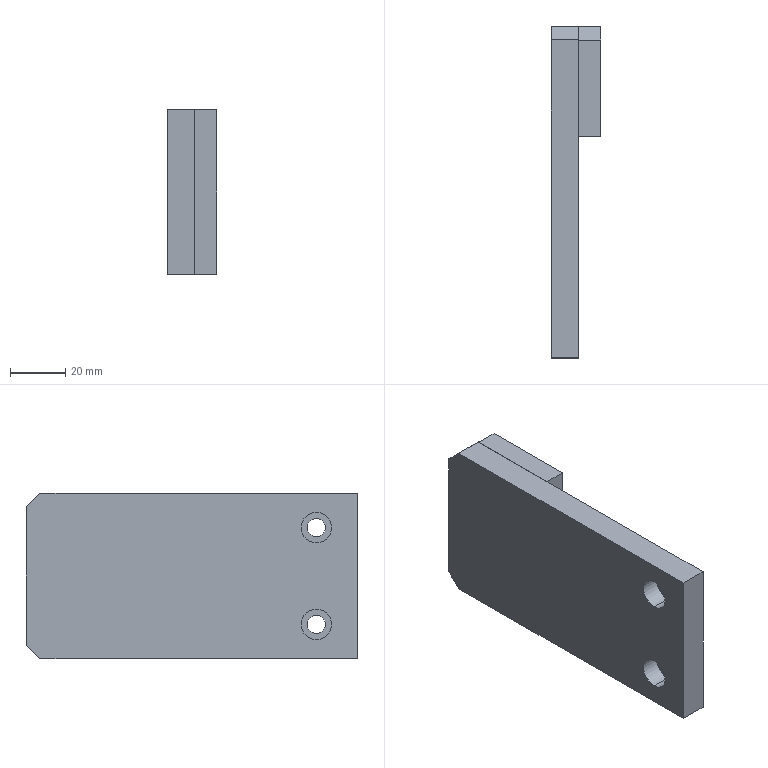Part | SolidWorks | features BaseBody 1 | 1 solid | 25 faces | box 18 x 120 x 60 mm | volume 89024 mm3 | plane 17 | cylinder 8 | commonest cylinder face diameters 6.6 x4 11 x4
STEP:
#1=CARTESIAN_POINT('',(6.8,15.,-23.));
#2=VERTEX_POINT('',#1);
#3=CARTESIAN_POINT('',(6.8,15.,-12.));
#4=VERTEX_POINT('',#3);
#5=CARTESIAN_POINT('',(6.8,15.,-17.5));
#6=DIRECTION('',(-1.,0.,0.));
#7=DIRECTION('',(0.,0.,1.));
#8=AXIS2_PLACEMENT_3D('',#5,#6,#7);
#9=CIRCLE('',#8,5.5);
#10=EDGE_CURVE('',#2,#4,#9,.T.);
#11=ORIENTED_EDGE('',*,*,#10,.F.);
#12=CARTESIAN_POINT('',(0.,15.,-23.));
#13=VERTEX_POINT('',#12);
#14=CARTESIAN_POINT('',(0.,15.,-23.));
#15=DIRECTION('',(-1.,0.,0.));
#16=VECTOR('',#15,1000.);
#17=LINE('',#14,#16);
#18=EDGE_CURVE('',#2,#13,#17,.T.);
#19=ORIENTED_EDGE('',*,*,#18,.T.);
#20=CARTESIAN_POINT('',(0.,15.,-12.));
#21=VERTEX_POINT('',#20);
#22=CARTESIAN_POINT('',(0.,15.,-17.5));
#23=DIRECTION('',(-1.,0.,0.));
#24=DIRECTION('',(0.,0.,1.));
#25=AXIS2_PLACEMENT_3D('',#22,#23,#24);
#26=CIRCLE('',#25,5.5);
#27=EDGE_CURVE('',#13,#21,#26,.T.);
#28=ORIENTED_EDGE('',*,*,#27,.T.);
#29=CARTESIAN_POINT('',(0.,15.,-12.));
#30=DIRECTION('',(-1.,0.,0.));
#31=VECTOR('',#30,1000.);
#32=LINE('',#29,#31);
#33=EDGE_CURVE('',#4,#21,#32,.T.);
#34=ORIENTED_EDGE('',*,*,#33,.F.);
#35=EDGE_LOOP('',(#11,#19,#28,#34));
#36=FACE_OUTER_BOUND('',#35,.T.);
#37=CARTESIAN_POINT('',(0.,15.,-17.5));
#38=DIRECTION('',(-1.,0.,0.));
#39=DIRECTION('',(0.,0.,1.));
#40=AXIS2_PLACEMENT_3D('',#37,#38,#39);
#41=CYLINDRICAL_SURFACE('',#40,5.5);
#42=ADVANCED_FACE('',(#36),#41,.F.);
#43=CARTESIAN_POINT('',(10.,15.,-20.8));
#44=VERTEX_POINT('',#43);
#45=CARTESIAN_POINT('',(10.,15.,-14.2));
#46=VERTEX_POINT('',#45);
#47=CARTESIAN_POINT('',(10.,15.,-17.5));
#48=DIRECTION('',(-1.,0.,0.));
#49=DIRECTION('',(0.,0.,1.));
#50=AXIS2_PLACEMENT_3D('',#47,#48,#49);
#51=CIRCLE('',#50,3.3);
#52=EDGE_CURVE('',#44,#46,#51,.T.);
#53=ORIENTED_EDGE('',*,*,#52,.F.);
#54=CARTESIAN_POINT('',(6.8,15.,-20.8));
#55=VERTEX_POINT('',#54);
#56=CARTESIAN_POINT('',(0.,15.,-20.8));
#57=DIRECTION('',(-1.,0.,0.));
#58=VECTOR('',#57,1000.);
#59=LINE('',#56,#58);
#60=EDGE_CURVE('',#44,#55,#59,.T.);
#61=ORIENTED_EDGE('',*,*,#60,.T.);
#62=CARTESIAN_POINT('',(6.8,15.,-14.2));
#63=VERTEX_POINT('',#62);
#64=CARTESIAN_POINT('',(6.8,15.,-17.5));
#65=DIRECTION('',(-1.,0.,0.));
#66=DIRECTION('',(0.,0.,1.));
#67=AXIS2_PLACEMENT_3D('',#64,#65,#66);
#68=CIRCLE('',#67,3.3);
#69=EDGE_CURVE('',#55,#63,#68,.T.);
#70=ORIENTED_EDGE('',*,*,#69,.T.);
#71=CARTESIAN_POINT('',(0.,15.,-14.2));
#72=DIRECTION('',(-1.,0.,0.));
#73=VECTOR('',#72,1000.);
#74=LINE('',#71,#73);
#75=EDGE_CURVE('',#46,#63,#74,.T.);
#76=ORIENTED_EDGE('',*,*,#75,.F.);
#77=EDGE_LOOP('',(#53,#61,#70,#76));
#78=FACE_OUTER_BOUND('',#77,.T.);
#79=CARTESIAN_POINT('',(0.,15.,-17.5));
#80=DIRECTION('',(-1.,0.,0.));
#81=DIRECTION('',(0.,0.,1.));
#82=AXIS2_PLACEMENT_3D('',#79,#80,#81);
#83=CYLINDRICAL_SURFACE('',#82,3.3);
#84=ADVANCED_FACE('',(#78),#83,.F.);
#85=CARTESIAN_POINT('',(6.8,15.,12.));
#86=VERTEX_POINT('',#85);
#87=CARTESIAN_POINT('',(6.8,15.,23.));
#88=VERTEX_POINT('',#87);
#89=CARTESIAN_POINT('',(6.8,15.,17.5));
#90=DIRECTION('',(-1.,0.,0.));
#91=DIRECTION('',(0.,0.,1.));
#92=AXIS2_PLACEMENT_3D('',#89,#90,#91);
#93=CIRCLE('',#92,5.5);
#94=EDGE_CURVE('',#86,#88,#93,.T.);
#95=ORIENTED_EDGE('',*,*,#94,.F.);
#96=CARTESIAN_POINT('',(0.,15.,12.));
#97=VERTEX_POINT('',#96);
#98=CARTESIAN_POINT('',(0.,15.,12.));
#99=DIRECTION('',(-1.,0.,0.));
#100=VECTOR('',#99,1000.);
#101=LINE('',#98,#100);
#102=EDGE_CURVE('',#86,#97,#101,.T.);
#103=ORIENTED_EDGE('',*,*,#102,.T.);
#104=CARTESIAN_POINT('',(0.,15.,23.));
#105=VERTEX_POINT('',#104);
#106=CARTESIAN_POINT('',(0.,15.,17.5));
#107=DIRECTION('',(-1.,0.,0.));
#108=DIRECTION('',(0.,0.,1.));
#109=AXIS2_PLACEMENT_3D('',#106,#107,#108);
#110=CIRCLE('',#109,5.5);
#111=EDGE_CURVE('',#97,#105,#110,.T.);
#112=ORIENTED_EDGE('',*,*,#111,.T.);
#113=CARTESIAN_POINT('',(0.,15.,23.));
#114=DIRECTION('',(-1.,0.,0.));
#115=VECTOR('',#114,1000.);
#116=LINE('',#113,#115);
#117=EDGE_CURVE('',#88,#105,#116,.T.);
#118=ORIENTED_EDGE('',*,*,#117,.F.);
#119=EDGE_LOOP('',(#95,#103,#112,#118));
#120=FACE_OUTER_BOUND('',#119,.T.);
#121=CARTESIAN_POINT('',(0.,15.,17.5));
#122=DIRECTION('',(-1.,0.,0.));
#123=DIRECTION('',(0.,0.,1.));
#124=AXIS2_PLACEMENT_3D('',#121,#122,#123);
#125=CYLINDRICAL_SURFACE('',#124,5.5);
#126=ADVANCED_FACE('',(#120),#125,.F.);
#127=CARTESIAN_POINT('',(10.,15.,14.2));
#128=VERTEX_POINT('',#127);
#129=CARTESIAN_POINT('',(10.,15.,20.8));
#130=VERTEX_POINT('',#129);
#131=CARTESIAN_POINT('',(10.,15.,17.5));
#132=DIRECTION('',(-1.,0.,0.));
#133=DIRECTION('',(0.,0.,1.));
#134=AXIS2_PLACEMENT_3D('',#131,#132,#133);
#135=CIRCLE('',#134,3.3);
#136=EDGE_CURVE('',#128,#130,#135,.T.);
#137=ORIENTED_EDGE('',*,*,#136,.F.);
#138=CARTESIAN_POINT('',(6.8,15.,14.2));
#139=VERTEX_POINT('',#138);
#140=CARTESIAN_POINT('',(0.,15.,14.2));
#141=DIRECTION('',(-1.,0.,0.));
#142=VECTOR('',#141,1000.);
#143=LINE('',#140,#142);
#144=EDGE_CURVE('',#128,#139,#143,.T.);
#145=ORIENTED_EDGE('',*,*,#144,.T.);
#146=CARTESIAN_POINT('',(6.8,15.,20.8));
#147=VERTEX_POINT('',#146);
#148=CARTESIAN_POINT('',(6.8,15.,17.5));
#149=DIRECTION('',(-1.,0.,0.));
#150=DIRECTION('',(0.,0.,1.));
#151=AXIS2_PLACEMENT_3D('',#148,#149,#150);
#152=CIRCLE('',#151,3.3);
#153=EDGE_CURVE('',#139,#147,#152,.T.);
#154=ORIENTED_EDGE('',*,*,#153,.T.);
#155=CARTESIAN_POINT('',(0.,15.,20.8));
#156=DIRECTION('',(-1.,0.,0.));
#157=VECTOR('',#156,1000.);
#158=LINE('',#155,#157);
#159=EDGE_CURVE('',#130,#147,#158,.T.);
#160=ORIENTED_EDGE('',*,*,#159,.F.);
#161=EDGE_LOOP('',(#137,#145,#154,#160));
#162=FACE_OUTER_BOUND('',#161,.T.);
#163=CARTESIAN_POINT('',(0.,15.,17.5));
#164=DIRECTION('',(-1.,0.,0.));
#165=DIRECTION('',(0.,0.,1.));
#166=AXIS2_PLACEMENT_3D('',#163,#164,#165);
#167=CYLINDRICAL_SURFACE('',#166,3.3);
#168=ADVANCED_FACE('',(#162),#167,.F.);
#169=CARTESIAN_POINT('',(18.,114.917,29.8));
#170=VERTEX_POINT('',#169);
#171=CARTESIAN_POINT('',(18.,80.,29.8));
#172=VERTEX_POINT('',#171);
#173=CARTESIAN_POINT('',(18.,114.917,29.8));
#174=DIRECTION('',(0.,-1.,0.));
#175=VECTOR('',#174,1000.);
#176=LINE('',#173,#175);
#177=EDGE_CURVE('',#170,#172,#176,.T.);
#178=ORIENTED_EDGE('',*,*,#177,.T.);
#179=CARTESIAN_POINT('',(18.,80.,-29.8));
#180=VERTEX_POINT('',#179);
#181=CARTESIAN_POINT('',(18.,80.,29.8));
#182=DIRECTION('',(0.,0.,-1.));
#183=VECTOR('',#182,1000.);
#184=LINE('',#181,#183);
#185=EDGE_CURVE('',#172,#180,#184,.T.);
#186=ORIENTED_EDGE('',*,*,#185,.T.);
#187=CARTESIAN_POINT('',(18.,114.917,-29.8));
#188=VERTEX_POINT('',#187);
#189=CARTESIAN_POINT('',(18.,80.,-29.8));
#190=DIRECTION('',(0.,1.,0.));
#191=VECTOR('',#190,1000.);
#192=LINE('',#189,#191);
#193=EDGE_CURVE('',#180,#188,#192,.T.);
#194=ORIENTED_EDGE('',*,*,#193,.T.);
#195=CARTESIAN_POINT('',(18.,119.8,-24.917));
#196=VERTEX_POINT('',#195);
#197=CARTESIAN_POINT('',(18.,114.917,-29.8));
#198=DIRECTION('',(0.,0.7071,0.7071));
#199=VECTOR('',#198,1000.);
#200=LINE('',#197,#199);
#201=EDGE_CURVE('',#188,#196,#200,.T.);
#202=ORIENTED_EDGE('',*,*,#201,.T.);
#203=CARTESIAN_POINT('',(18.,119.8,24.917));
#204=VERTEX_POINT('',#203);
#205=CARTESIAN_POINT('',(18.,119.8,-24.917));
#206=DIRECTION('',(0.,0.,1.));
#207=VECTOR('',#206,1000.);
#208=LINE('',#205,#207);
#209=EDGE_CURVE('',#196,#204,#208,.T.);
#210=ORIENTED_EDGE('',*,*,#209,.T.);
#211=CARTESIAN_POINT('',(18.,119.8,24.917));
#212=DIRECTION('',(0.,-0.7071,0.7071));
#213=VECTOR('',#212,1000.);
#214=LINE('',#211,#213);
#215=EDGE_CURVE('',#204,#170,#214,.T.);
#216=ORIENTED_EDGE('',*,*,#215,.T.);
#217=EDGE_LOOP('',(#178,#186,#194,#202,#210,#216));
#218=FACE_OUTER_BOUND('',#217,.T.);
#219=CARTESIAN_POINT('',(18.,0.,0.));
#220=DIRECTION('',(1.,0.,0.));
#221=DIRECTION('',(0.,1.,0.));
#222=AXIS2_PLACEMENT_3D('',#219,#220,#221);
#223=PLANE('',#222);
#224=ADVANCED_FACE('',(#218),#223,.T.);
#225=CARTESIAN_POINT('',(10.,119.8,24.917));
#226=VERTEX_POINT('',#225);
#227=CARTESIAN_POINT('',(10.,114.917,29.8));
#228=VERTEX_POINT('',#227);
#229=CARTESIAN_POINT('',(10.,119.8,24.917));
#230=DIRECTION('',(0.,-0.7071,0.7071));
#231=VECTOR('',#230,1000.);
#232=LINE('',#229,#231);
#233=EDGE_CURVE('',#226,#228,#232,.T.);
#234=ORIENTED_EDGE('',*,*,#233,.T.);
#235=CARTESIAN_POINT('',(18.,114.917,29.8));
#236=DIRECTION('',(-1.,0.,0.));
#237=VECTOR('',#236,1000.);
#238=LINE('',#235,#237);
#239=EDGE_CURVE('',#170,#228,#238,.T.);
#240=ORIENTED_EDGE('',*,*,#239,.F.);
#241=ORIENTED_EDGE('',*,*,#215,.F.);
#242=CARTESIAN_POINT('',(18.,119.8,24.917));
#243=DIRECTION('',(-1.,0.,0.));
#244=VECTOR('',#243,1000.);
#245=LINE('',#242,#244);
#246=EDGE_CURVE('',#204,#226,#245,.T.);
#247=ORIENTED_EDGE('',*,*,#246,.T.);
#248=EDGE_LOOP('',(#234,#240,#241,#247));
#249=FACE_OUTER_BOUND('',#248,.T.);
#250=CARTESIAN_POINT('',(18.,119.8,24.917));
#251=DIRECTION('',(0.,-0.7071,-0.7071));
#252=DIRECTION('',(0.,0.7071,-0.7071));
#253=AXIS2_PLACEMENT_3D('',#250,#251,#252);
#254=PLANE('',#253);
#255=ADVANCED_FACE('',(#249),#254,.F.);
#256=CARTESIAN_POINT('',(10.,119.8,-24.917));
#257=VERTEX_POINT('',#256);
#258=CARTESIAN_POINT('',(10.,119.8,-24.917));
#259=DIRECTION('',(0.,0.,1.));
#260=VECTOR('',#259,1000.);
#261=LINE('',#258,#260);
#262=EDGE_CURVE('',#257,#226,#261,.T.);
#263=ORIENTED_EDGE('',*,*,#262,.T.);
#264=ORIENTED_EDGE('',*,*,#246,.F.);
#265=ORIENTED_EDGE('',*,*,#209,.F.);
#266=CARTESIAN_POINT('',(18.,119.8,-24.917));
#267=DIRECTION('',(-1.,0.,0.));
#268=VECTOR('',#267,1000.);
#269=LINE('',#266,#268);
#270=EDGE_CURVE('',#196,#257,#269,.T.);
#271=ORIENTED_EDGE('',*,*,#270,.T.);
#272=EDGE_LOOP('',(#263,#264,#265,#271));
#273=FACE_OUTER_BOUND('',#272,.T.);
#274=CARTESIAN_POINT('',(18.,119.8,-24.917));
#275=DIRECTION('',(0.,-1.,0.));
#276=DIRECTION('',(0.,0.,-1.));
#277=AXIS2_PLACEMENT_3D('',#274,#275,#276);
#278=PLANE('',#277);
#279=ADVANCED_FACE('',(#273),#278,.F.);
#280=CARTESIAN_POINT('',(10.,114.917,-29.8));
#281=VERTEX_POINT('',#280);
#282=CARTESIAN_POINT('',(10.,114.917,-29.8));
#283=DIRECTION('',(0.,0.7071,0.7071));
#284=VECTOR('',#283,1000.);
#285=LINE('',#282,#284);
#286=EDGE_CURVE('',#281,#257,#285,.T.);
#287=ORIENTED_EDGE('',*,*,#286,.T.);
#288=ORIENTED_EDGE('',*,*,#270,.F.);
#289=ORIENTED_EDGE('',*,*,#201,.F.);
#290=CARTESIAN_POINT('',(18.,114.917,-29.8));
#291=DIRECTION('',(-1.,0.,0.));
#292=VECTOR('',#291,1000.);
#293=LINE('',#290,#292);
#294=EDGE_CURVE('',#188,#281,#293,.T.);
#295=ORIENTED_EDGE('',*,*,#294,.T.);
#296=EDGE_LOOP('',(#287,#288,#289,#295));
#297=FACE_OUTER_BOUND('',#296,.T.);
#298=CARTESIAN_POINT('',(18.,114.917,-29.8));
#299=DIRECTION('',(0.,-0.7071,0.7071));
#300=DIRECTION('',(-1.,0.,0.));
#301=AXIS2_PLACEMENT_3D('',#298,#299,#300);
#302=PLANE('',#301);
#303=ADVANCED_FACE('',(#297),#302,.F.);
#304=CARTESIAN_POINT('',(10.,80.,-29.8));
#305=VERTEX_POINT('',#304);
#306=CARTESIAN_POINT('',(10.,80.,-29.8));
#307=DIRECTION('',(0.,1.,0.));
#308=VECTOR('',#307,1000.);
#309=LINE('',#306,#308);
#310=EDGE_CURVE('',#305,#281,#309,.T.);
#311=ORIENTED_EDGE('',*,*,#310,.T.);
#312=ORIENTED_EDGE('',*,*,#294,.F.);
#313=ORIENTED_EDGE('',*,*,#193,.F.);
#314=CARTESIAN_POINT('',(18.,80.,-29.8));
#315=DIRECTION('',(-1.,0.,0.));
#316=VECTOR('',#315,1000.);
#317=LINE('',#314,#316);
#318=EDGE_CURVE('',#180,#305,#317,.T.);
#319=ORIENTED_EDGE('',*,*,#318,.T.);
#320=EDGE_LOOP('',(#311,#312,#313,#319));
#321=FACE_OUTER_BOUND('',#320,.T.);
#322=CARTESIAN_POINT('',(18.,80.,-29.8));
#323=DIRECTION('',(0.,0.,1.));
#324=DIRECTION('',(0.,-1.,0.));
#325=AXIS2_PLACEMENT_3D('',#322,#323,#324);
#326=PLANE('',#325);
#327=ADVANCED_FACE('',(#321),#326,.F.);
#328=CARTESIAN_POINT('',(10.,80.,29.8));
#329=VERTEX_POINT('',#328);
#330=CARTESIAN_POINT('',(10.,80.,29.8));
#331=DIRECTION('',(0.,0.,-1.));
#332=VECTOR('',#331,1000.);
#333=LINE('',#330,#332);
#334=EDGE_CURVE('',#329,#305,#333,.T.);
#335=ORIENTED_EDGE('',*,*,#334,.T.);
#336=ORIENTED_EDGE('',*,*,#318,.F.);
#337=ORIENTED_EDGE('',*,*,#185,.F.);
#338=CARTESIAN_POINT('',(18.,80.,29.8));
#339=DIRECTION('',(-1.,0.,0.));
#340=VECTOR('',#339,1000.);
#341=LINE('',#338,#340);
#342=EDGE_CURVE('',#172,#329,#341,.T.);
#343=ORIENTED_EDGE('',*,*,#342,.T.);
#344=EDGE_LOOP('',(#335,#336,#337,#343));
#345=FACE_OUTER_BOUND('',#344,.T.);
#346=CARTESIAN_POINT('',(18.,80.,29.8));
#347=DIRECTION('',(0.,1.,0.));
#348=DIRECTION('',(1.,0.,0.));
#349=AXIS2_PLACEMENT_3D('',#346,#347,#348);
#350=PLANE('',#349);
#351=ADVANCED_FACE('',(#345),#350,.F.);
#352=CARTESIAN_POINT('',(10.,114.917,29.8));
#353=DIRECTION('',(0.,-1.,0.));
#354=VECTOR('',#353,1000.);
#355=LINE('',#352,#354);
#356=EDGE_CURVE('',#228,#329,#355,.T.);
#357=ORIENTED_EDGE('',*,*,#356,.T.);
#358=ORIENTED_EDGE('',*,*,#342,.F.);
#359=ORIENTED_EDGE('',*,*,#177,.F.);
#360=ORIENTED_EDGE('',*,*,#239,.T.);
#361=EDGE_LOOP('',(#357,#358,#359,#360));
#362=FACE_OUTER_BOUND('',#361,.T.);
#363=CARTESIAN_POINT('',(18.,114.917,29.8));
#364=DIRECTION('',(0.,0.,-1.));
#365=DIRECTION('',(-1.,0.,0.));
#366=AXIS2_PLACEMENT_3D('',#363,#364,#365);
#367=PLANE('',#366);
#368=ADVANCED_FACE('',(#362),#367,.F.);
#369=CARTESIAN_POINT('',(10.,120.,25.));
#370=VERTEX_POINT('',#369);
#371=CARTESIAN_POINT('',(10.,115.,30.));
#372=VERTEX_POINT('',#371);
#373=CARTESIAN_POINT('',(10.,115.,30.));
#374=DIRECTION('',(0.,-0.7071,0.7071));
#375=VECTOR('',#374,1000.);
#376=LINE('',#373,#375);
#377=EDGE_CURVE('',#370,#372,#376,.T.);
#378=ORIENTED_EDGE('',*,*,#377,.F.);
#379=CARTESIAN_POINT('',(0.,120.,25.));
#380=VERTEX_POINT('',#379);
#381=CARTESIAN_POINT('',(10.,120.,25.));
#382=DIRECTION('',(1.,0.,0.));
#383=VECTOR('',#382,1000.);
#384=LINE('',#381,#383);
#385=EDGE_CURVE('',#380,#370,#384,.T.);
#386=ORIENTED_EDGE('',*,*,#385,.F.);
#387=CARTESIAN_POINT('',(0.,115.,30.));
#388=VERTEX_POINT('',#387);
#389=CARTESIAN_POINT('',(0.,72.5,72.5));
#390=DIRECTION('',(0.,0.7071,-0.7071));
#391=VECTOR('',#390,1000.);
#392=LINE('',#389,#391);
#393=EDGE_CURVE('',#388,#380,#392,.T.);
#394=ORIENTED_EDGE('',*,*,#393,.F.);
#395=CARTESIAN_POINT('',(10.,115.,30.));
#396=DIRECTION('',(-1.,0.,0.));
#397=VECTOR('',#396,1000.);
#398=LINE('',#395,#397);
#399=EDGE_CURVE('',#372,#388,#398,.T.);
#400=ORIENTED_EDGE('',*,*,#399,.F.);
#401=EDGE_LOOP('',(#378,#386,#394,#400));
#402=FACE_OUTER_BOUND('',#401,.T.);
#403=CARTESIAN_POINT('',(10.,115.,30.));
#404=DIRECTION('',(0.,-0.7071,-0.7071));
#405=DIRECTION('',(0.,0.7071,-0.7071));
#406=AXIS2_PLACEMENT_3D('',#403,#404,#405);
#407=PLANE('',#406);
#408=ADVANCED_FACE('',(#402),#407,.F.);
#409=CARTESIAN_POINT('',(10.,115.,-30.));
#410=VERTEX_POINT('',#409);
#411=CARTESIAN_POINT('',(10.,120.,-25.));
#412=VERTEX_POINT('',#411);
#413=CARTESIAN_POINT('',(10.,120.,-25.));
#414=DIRECTION('',(0.,0.7071,0.7071));
#415=VECTOR('',#414,1000.);
#416=LINE('',#413,#415);
#417=EDGE_CURVE('',#410,#412,#416,.T.);
#418=ORIENTED_EDGE('',*,*,#417,.F.);
#419=CARTESIAN_POINT('',(0.,115.,-30.));
#420=VERTEX_POINT('',#419);
#421=CARTESIAN_POINT('',(10.,115.,-30.));
#422=DIRECTION('',(1.,0.,0.));
#423=VECTOR('',#422,1000.);
#424=LINE('',#421,#423);
#425=EDGE_CURVE('',#420,#410,#424,.T.);
#426=ORIENTED_EDGE('',*,*,#425,.F.);
#427=CARTESIAN_POINT('',(0.,120.,-25.));
#428=VERTEX_POINT('',#427);
#429=CARTESIAN_POINT('',(0.,72.5,-72.5));
#430=DIRECTION('',(0.,-0.7071,-0.7071));
#431=VECTOR('',#430,1000.);
#432=LINE('',#429,#431);
#433=EDGE_CURVE('',#428,#420,#432,.T.);
#434=ORIENTED_EDGE('',*,*,#433,.F.);
#435=CARTESIAN_POINT('',(10.,120.,-25.));
#436=DIRECTION('',(-1.,0.,0.));
#437=VECTOR('',#436,1000.);
#438=LINE('',#435,#437);
#439=EDGE_CURVE('',#412,#428,#438,.T.);
#440=ORIENTED_EDGE('',*,*,#439,.F.);
#441=EDGE_LOOP('',(#418,#426,#434,#440));
#442=FACE_OUTER_BOUND('',#441,.T.);
#443=CARTESIAN_POINT('',(10.,120.,-25.));
#444=DIRECTION('',(0.,-0.7071,0.7071));
#445=DIRECTION('',(-1.,0.,0.));
#446=AXIS2_PLACEMENT_3D('',#443,#444,#445);
#447=PLANE('',#446);
#448=ADVANCED_FACE('',(#442),#447,.F.);
#449=CARTESIAN_POINT('',(6.8,15.,-17.5));
#450=DIRECTION('',(-1.,0.,0.));
#451=DIRECTION('',(0.,0.,1.));
#452=AXIS2_PLACEMENT_3D('',#449,#450,#451);
#453=CIRCLE('',#452,3.3);
#454=EDGE_CURVE('',#63,#55,#453,.T.);
#455=ORIENTED_EDGE('',*,*,#454,.F.);
#456=ORIENTED_EDGE('',*,*,#69,.F.);
#457=EDGE_LOOP('',(#455,#456));
#458=FACE_BOUND('',#457,.T.);
#459=CARTESIAN_POINT('',(6.8,15.,-17.5));
#460=DIRECTION('',(-1.,0.,0.));
#461=DIRECTION('',(0.,0.,1.));
#462=AXIS2_PLACEMENT_3D('',#459,#460,#461);
#463=CIRCLE('',#462,5.5);
#464=EDGE_CURVE('',#4,#2,#463,.T.);
#465=ORIENTED_EDGE('',*,*,#464,.T.);
#466=ORIENTED_EDGE('',*,*,#10,.T.);
#467=EDGE_LOOP('',(#465,#466));
#468=FACE_OUTER_BOUND('',#467,.T.);
#469=CARTESIAN_POINT('',(6.8,18.3,-17.5));
#470=DIRECTION('',(1.,0.,0.));
#471=DIRECTION('',(0.,1.,0.));
#472=AXIS2_PLACEMENT_3D('',#469,#470,#471);
#473=PLANE('',#472);
#474=ADVANCED_FACE('',(#458,#468),#473,.F.);
#475=CARTESIAN_POINT('',(6.8,15.,17.5));
#476=DIRECTION('',(-1.,0.,0.));
#477=DIRECTION('',(0.,0.,1.));
#478=AXIS2_PLACEMENT_3D('',#475,#476,#477);
#479=CIRCLE('',#478,3.3);
#480=EDGE_CURVE('',#147,#139,#479,.T.);
#481=ORIENTED_EDGE('',*,*,#480,.F.);
#482=ORIENTED_EDGE('',*,*,#153,.F.);
#483=EDGE_LOOP('',(#481,#482));
#484=FACE_BOUND('',#483,.T.);
#485=CARTESIAN_POINT('',(6.8,15.,17.5));
#486=DIRECTION('',(-1.,0.,0.));
#487=DIRECTION('',(0.,0.,1.));
#488=AXIS2_PLACEMENT_3D('',#485,#486,#487);
#489=CIRCLE('',#488,5.5);
#490=EDGE_CURVE('',#88,#86,#489,.T.);
#491=ORIENTED_EDGE('',*,*,#490,.T.);
#492=ORIENTED_EDGE('',*,*,#94,.T.);
#493=EDGE_LOOP('',(#491,#492));
#494=FACE_OUTER_BOUND('',#493,.T.);
#495=CARTESIAN_POINT('',(6.8,18.3,17.5));
#496=DIRECTION('',(1.,0.,0.));
#497=DIRECTION('',(0.,1.,0.));
#498=AXIS2_PLACEMENT_3D('',#495,#496,#497);
#499=PLANE('',#498);
#500=ADVANCED_FACE('',(#484,#494),#499,.F.);
#501=CARTESIAN_POINT('',(0.,15.,17.5));
#502=DIRECTION('',(-1.,0.,0.));
#503=DIRECTION('',(0.,0.,1.));
#504=AXIS2_PLACEMENT_3D('',#501,#502,#503);
#505=CIRCLE('',#504,5.5);
#506=EDGE_CURVE('',#105,#97,#505,.T.);
#507=ORIENTED_EDGE('',*,*,#506,.F.);
#508=ORIENTED_EDGE('',*,*,#111,.F.);
#509=EDGE_LOOP('',(#507,#508));
#510=FACE_BOUND('',#509,.T.);
#511=CARTESIAN_POINT('',(0.,15.,-17.5));
#512=DIRECTION('',(-1.,0.,0.));
#513=DIRECTION('',(0.,0.,1.));
#514=AXIS2_PLACEMENT_3D('',#511,#512,#513);
#515=CIRCLE('',#514,5.5);
#516=EDGE_CURVE('',#21,#13,#515,.T.);
#517=ORIENTED_EDGE('',*,*,#516,.F.);
#518=ORIENTED_EDGE('',*,*,#27,.F.);
#519=EDGE_LOOP('',(#517,#518));
#520=FACE_BOUND('',#519,.T.);
#521=CARTESIAN_POINT('',(0.,120.,30.));
#522=DIRECTION('',(0.,0.,1.));
#523=VECTOR('',#522,1000.);
#524=LINE('',#521,#523);
#525=EDGE_CURVE('',#428,#380,#524,.T.);
#526=ORIENTED_EDGE('',*,*,#525,.F.);
#527=ORIENTED_EDGE('',*,*,#433,.T.);
#528=CARTESIAN_POINT('',(0.,0.,-30.));
#529=VERTEX_POINT('',#528);
#530=CARTESIAN_POINT('',(0.,0.,-30.));
#531=DIRECTION('',(0.,1.,0.));
#532=VECTOR('',#531,1000.);
#533=LINE('',#530,#532);
#534=EDGE_CURVE('',#529,#420,#533,.T.);
#535=ORIENTED_EDGE('',*,*,#534,.F.);
#536=CARTESIAN_POINT('',(0.,0.,30.));
#537=VERTEX_POINT('',#536);
#538=CARTESIAN_POINT('',(0.,0.,30.));
#539=DIRECTION('',(0.,0.,-1.));
#540=VECTOR('',#539,1000.);
#541=LINE('',#538,#540);
#542=EDGE_CURVE('',#537,#529,#541,.T.);
#543=ORIENTED_EDGE('',*,*,#542,.F.);
#544=CARTESIAN_POINT('',(0.,0.,30.));
#545=DIRECTION('',(0.,-1.,0.));
#546=VECTOR('',#545,1000.);
#547=LINE('',#544,#546);
#548=EDGE_CURVE('',#388,#537,#547,.T.);
#549=ORIENTED_EDGE('',*,*,#548,.F.);
#550=ORIENTED_EDGE('',*,*,#393,.T.);
#551=EDGE_LOOP('',(#526,#527,#535,#543,#549,#550));
#552=FACE_OUTER_BOUND('',#551,.T.);
#553=CARTESIAN_POINT('',(0.,0.,0.));
#554=DIRECTION('',(-1.,0.,0.));
#555=DIRECTION('',(0.,0.,1.));
#556=AXIS2_PLACEMENT_3D('',#553,#554,#555);
#557=PLANE('',#556);
#558=ADVANCED_FACE('',(#510,#520,#552),#557,.T.);
#559=CARTESIAN_POINT('',(10.,120.,30.));
#560=DIRECTION('',(0.,0.,1.));
#561=VECTOR('',#560,1000.);
#562=LINE('',#559,#561);
#563=EDGE_CURVE('',#412,#370,#562,.T.);
#564=ORIENTED_EDGE('',*,*,#563,.F.);
#565=ORIENTED_EDGE('',*,*,#439,.T.);
#566=ORIENTED_EDGE('',*,*,#525,.T.);
#567=ORIENTED_EDGE('',*,*,#385,.T.);
#568=EDGE_LOOP('',(#564,#565,#566,#567));
#569=FACE_OUTER_BOUND('',#568,.T.);
#570=CARTESIAN_POINT('',(10.,120.,30.));
#571=DIRECTION('',(0.,-1.,0.));
#572=DIRECTION('',(0.,0.,-1.));
#573=AXIS2_PLACEMENT_3D('',#570,#571,#572);
#574=PLANE('',#573);
#575=ADVANCED_FACE('',(#569),#574,.F.);
#576=ORIENTED_EDGE('',*,*,#534,.T.);
#577=ORIENTED_EDGE('',*,*,#425,.T.);
#578=CARTESIAN_POINT('',(10.,0.,-30.));
#579=VERTEX_POINT('',#578);
#580=CARTESIAN_POINT('',(10.,0.,-30.));
#581=DIRECTION('',(0.,1.,0.));
#582=VECTOR('',#581,1000.);
#583=LINE('',#580,#582);
#584=EDGE_CURVE('',#579,#410,#583,.T.);
#585=ORIENTED_EDGE('',*,*,#584,.F.);
#586=CARTESIAN_POINT('',(10.,0.,-30.));
#587=DIRECTION('',(-1.,0.,0.));
#588=VECTOR('',#587,1000.);
#589=LINE('',#586,#588);
#590=EDGE_CURVE('',#579,#529,#589,.T.);
#591=ORIENTED_EDGE('',*,*,#590,.T.);
#592=EDGE_LOOP('',(#576,#577,#585,#591));
#593=FACE_OUTER_BOUND('',#592,.T.);
#594=CARTESIAN_POINT('',(10.,0.,-30.));
#595=DIRECTION('',(0.,0.,1.));
#596=DIRECTION('',(1.,0.,0.));
#597=AXIS2_PLACEMENT_3D('',#594,#595,#596);
#598=PLANE('',#597);
#599=ADVANCED_FACE('',(#593),#598,.F.);
#600=ORIENTED_EDGE('',*,*,#542,.T.);
#601=ORIENTED_EDGE('',*,*,#590,.F.);
#602=CARTESIAN_POINT('',(10.,0.,30.));
#603=VERTEX_POINT('',#602);
#604=CARTESIAN_POINT('',(10.,0.,30.));
#605=DIRECTION('',(0.,0.,-1.));
#606=VECTOR('',#605,1000.);
#607=LINE('',#604,#606);
#608=EDGE_CURVE('',#603,#579,#607,.T.);
#609=ORIENTED_EDGE('',*,*,#608,.F.);
#610=CARTESIAN_POINT('',(10.,0.,30.));
#611=DIRECTION('',(-1.,0.,0.));
#612=VECTOR('',#611,1000.);
#613=LINE('',#610,#612);
#614=EDGE_CURVE('',#603,#537,#613,.T.);
#615=ORIENTED_EDGE('',*,*,#614,.T.);
#616=EDGE_LOOP('',(#600,#601,#609,#615));
#617=FACE_OUTER_BOUND('',#616,.T.);
#618=CARTESIAN_POINT('',(10.,0.,30.));
#619=DIRECTION('',(0.,1.,0.));
#620=DIRECTION('',(1.,0.,0.));
#621=AXIS2_PLACEMENT_3D('',#618,#619,#620);
#622=PLANE('',#621);
#623=ADVANCED_FACE('',(#617),#622,.F.);
#624=CARTESIAN_POINT('',(10.,0.,30.));
#625=DIRECTION('',(0.,-1.,0.));
#626=VECTOR('',#625,1000.);
#627=LINE('',#624,#626);
#628=EDGE_CURVE('',#372,#603,#627,.T.);
#629=ORIENTED_EDGE('',*,*,#628,.F.);
#630=ORIENTED_EDGE('',*,*,#399,.T.);
#631=ORIENTED_EDGE('',*,*,#548,.T.);
#632=ORIENTED_EDGE('',*,*,#614,.F.);
#633=EDGE_LOOP('',(#629,#630,#631,#632));
#634=FACE_OUTER_BOUND('',#633,.T.);
#635=CARTESIAN_POINT('',(10.,0.,30.));
#636=DIRECTION('',(0.,0.,-1.));
#637=DIRECTION('',(0.,-1.,0.));
#638=AXIS2_PLACEMENT_3D('',#635,#636,#637);
#639=PLANE('',#638);
#640=ADVANCED_FACE('',(#634),#639,.F.);
#641=ORIENTED_EDGE('',*,*,#356,.F.);
#642=ORIENTED_EDGE('',*,*,#233,.F.);
#643=ORIENTED_EDGE('',*,*,#262,.F.);
#644=ORIENTED_EDGE('',*,*,#286,.F.);
#645=ORIENTED_EDGE('',*,*,#310,.F.);
#646=ORIENTED_EDGE('',*,*,#334,.F.);
#647=EDGE_LOOP('',(#641,#642,#643,#644,#645,#646));
#648=FACE_BOUND('',#647,.T.);
#649=CARTESIAN_POINT('',(10.,15.,-17.5));
#650=DIRECTION('',(-1.,0.,0.));
#651=DIRECTION('',(0.,0.,1.));
#652=AXIS2_PLACEMENT_3D('',#649,#650,#651);
#653=CIRCLE('',#652,3.3);
#654=EDGE_CURVE('',#46,#44,#653,.T.);
#655=ORIENTED_EDGE('',*,*,#654,.T.);
#656=ORIENTED_EDGE('',*,*,#52,.T.);
#657=EDGE_LOOP('',(#655,#656));
#658=FACE_BOUND('',#657,.T.);
#659=CARTESIAN_POINT('',(10.,15.,17.5));
#660=DIRECTION('',(-1.,0.,0.));
#661=DIRECTION('',(0.,0.,1.));
#662=AXIS2_PLACEMENT_3D('',#659,#660,#661);
#663=CIRCLE('',#662,3.3);
#664=EDGE_CURVE('',#130,#128,#663,.T.);
#665=ORIENTED_EDGE('',*,*,#664,.T.);
#666=ORIENTED_EDGE('',*,*,#136,.T.);
#667=EDGE_LOOP('',(#665,#666));
#668=FACE_BOUND('',#667,.T.);
#669=ORIENTED_EDGE('',*,*,#584,.T.);
#670=ORIENTED_EDGE('',*,*,#417,.T.);
#671=ORIENTED_EDGE('',*,*,#563,.T.);
#672=ORIENTED_EDGE('',*,*,#377,.T.);
#673=ORIENTED_EDGE('',*,*,#628,.T.);
#674=ORIENTED_EDGE('',*,*,#608,.T.);
#675=EDGE_LOOP('',(#669,#670,#671,#672,#673,#674));
#676=FACE_OUTER_BOUND('',#675,.T.);
#677=CARTESIAN_POINT('',(10.,0.,0.));
#678=DIRECTION('',(-1.,0.,0.));
#679=DIRECTION('',(0.,0.,1.));
#680=AXIS2_PLACEMENT_3D('',#677,#678,#679);
#681=PLANE('',#680);
#682=ADVANCED_FACE('',(#648,#658,#668,#676),#681,.F.);
#683=ORIENTED_EDGE('',*,*,#144,.F.);
#684=ORIENTED_EDGE('',*,*,#664,.F.);
#685=ORIENTED_EDGE('',*,*,#159,.T.);
#686=ORIENTED_EDGE('',*,*,#480,.T.);
#687=EDGE_LOOP('',(#683,#684,#685,#686));
#688=FACE_OUTER_BOUND('',#687,.T.);
#689=CARTESIAN_POINT('',(0.,15.,17.5));
#690=DIRECTION('',(-1.,0.,0.));
#691=DIRECTION('',(0.,0.,1.));
#692=AXIS2_PLACEMENT_3D('',#689,#690,#691);
#693=CYLINDRICAL_SURFACE('',#692,3.3);
#694=ADVANCED_FACE('',(#688),#693,.F.);
#695=ORIENTED_EDGE('',*,*,#102,.F.);
#696=ORIENTED_EDGE('',*,*,#490,.F.);
#697=ORIENTED_EDGE('',*,*,#117,.T.);
#698=ORIENTED_EDGE('',*,*,#506,.T.);
#699=EDGE_LOOP('',(#695,#696,#697,#698));
#700=FACE_OUTER_BOUND('',#699,.T.);
#701=CARTESIAN_POINT('',(0.,15.,17.5));
#702=DIRECTION('',(-1.,0.,0.));
#703=DIRECTION('',(0.,0.,1.));
#704=AXIS2_PLACEMENT_3D('',#701,#702,#703);
#705=CYLINDRICAL_SURFACE('',#704,5.5);
#706=ADVANCED_FACE('',(#700),#705,.F.);
#707=ORIENTED_EDGE('',*,*,#60,.F.);
#708=ORIENTED_EDGE('',*,*,#654,.F.);
#709=ORIENTED_EDGE('',*,*,#75,.T.);
#710=ORIENTED_EDGE('',*,*,#454,.T.);
#711=EDGE_LOOP('',(#707,#708,#709,#710));
#712=FACE_OUTER_BOUND('',#711,.T.);
#713=CARTESIAN_POINT('',(0.,15.,-17.5));
#714=DIRECTION('',(-1.,0.,0.));
#715=DIRECTION('',(0.,0.,1.));
#716=AXIS2_PLACEMENT_3D('',#713,#714,#715);
#717=CYLINDRICAL_SURFACE('',#716,3.3);
#718=ADVANCED_FACE('',(#712),#717,.F.);
#719=ORIENTED_EDGE('',*,*,#18,.F.);
#720=ORIENTED_EDGE('',*,*,#464,.F.);
#721=ORIENTED_EDGE('',*,*,#33,.T.);
#722=ORIENTED_EDGE('',*,*,#516,.T.);
#723=EDGE_LOOP('',(#719,#720,#721,#722));
#724=FACE_OUTER_BOUND('',#723,.T.);
#725=CARTESIAN_POINT('',(0.,15.,-17.5));
#726=DIRECTION('',(-1.,0.,0.));
#727=DIRECTION('',(0.,0.,1.));
#728=AXIS2_PLACEMENT_3D('',#725,#726,#727);
#729=CYLINDRICAL_SURFACE('',#728,5.5);
#730=ADVANCED_FACE('',(#724),#729,.F.);
#731=CLOSED_SHELL('',(#42,#84,#126,#168,#224,#255,#279,#303,#327,#351,#368,#408,#448,#474,#500,#558,#575,#599,#623,#640,#682,#694,#706,#718,#730));
#732=MANIFOLD_SOLID_BREP('',#731);
#733=CARTESIAN_POINT('',(0.,0.,0.));
#734=DIRECTION('',(0.,0.,1.));
#735=DIRECTION('',(1.,0.,0.));
#736=AXIS2_PLACEMENT_3D('',#733,#734,#735);
#737=(LENGTH_UNIT()NAMED_UNIT(*)SI_UNIT(.MILLI.,.METRE.));
#738=UNCERTAINTY_MEASURE_WITH_UNIT(LENGTH_MEASURE(0.00001),#737,'','');
#739=(NAMED_UNIT(*)PLANE_ANGLE_UNIT()SI_UNIT($,.RADIAN.));
#740=(NAMED_UNIT(*)SI_UNIT($,.STERADIAN.)SOLID_ANGLE_UNIT());
#741=(GEOMETRIC_REPRESENTATION_CONTEXT(3)GLOBAL_UNCERTAINTY_ASSIGNED_CONTEXT((#738))GLOBAL_UNIT_ASSIGNED_CONTEXT((#737,#739,#740))REPRESENTATION_CONTEXT('',''));
#742=ADVANCED_BREP_SHAPE_REPRESENTATION('',(#732,#736),#741);